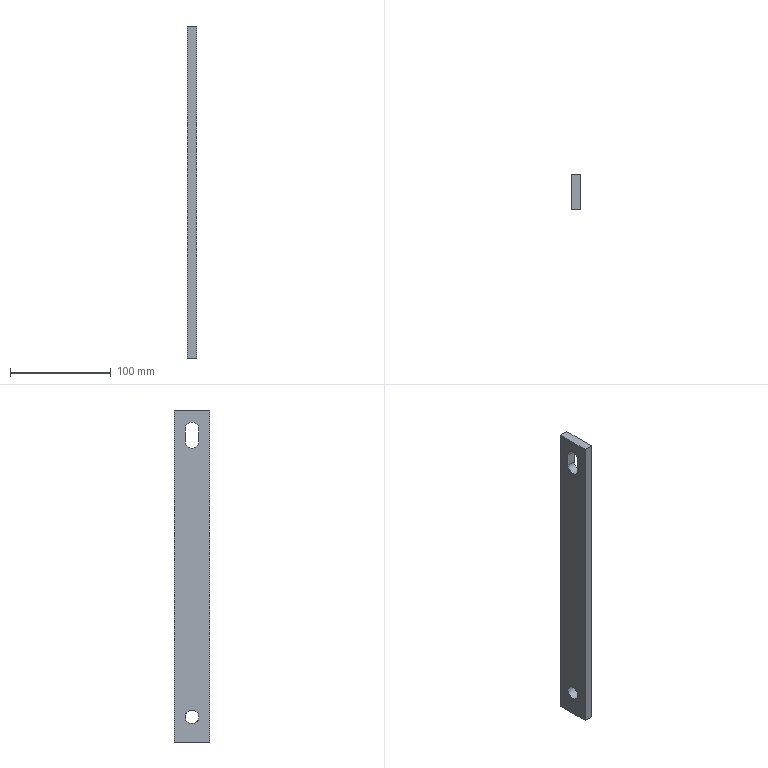Part | NX | features solid 2 | 1 solid | 11 faces | box 9 x 35 x 330 mm | volume 99855 mm3 | plane 8 | cylinder 3 | commonest cylinder face diameters 13.5 x3
STEP:
#1=CARTESIAN_POINT('',(1555.,-656.75,71.25));
#2=VERTEX_POINT('',#1);
#3=CARTESIAN_POINT('',(1555.,-643.25,71.25));
#4=VERTEX_POINT('',#3);
#5=CARTESIAN_POINT('',(1555.,-650.,71.25));
#6=DIRECTION('',(-1.,0.,0.));
#7=DIRECTION('',(0.,0.,-1.));
#8=AXIS2_PLACEMENT_3D('',#5,#6,#7);
#9=CIRCLE('',#8,6.75);
#10=EDGE_CURVE('',#2,#4,#9,.T.);
#11=ORIENTED_EDGE('',*,*,#10,.T.);
#12=CARTESIAN_POINT('',(1564.,-643.25,71.25));
#13=VERTEX_POINT('',#12);
#14=CARTESIAN_POINT('',(1558.,-643.25,71.25));
#15=DIRECTION('',(-1.,0.,0.));
#16=VECTOR('',#15,1000.);
#17=LINE('',#14,#16);
#18=EDGE_CURVE('',#13,#4,#17,.T.);
#19=ORIENTED_EDGE('',*,*,#18,.F.);
#20=CARTESIAN_POINT('',(1564.,-656.75,71.25));
#21=VERTEX_POINT('',#20);
#22=CARTESIAN_POINT('',(1564.,-650.,71.25));
#23=DIRECTION('',(-1.,0.,0.));
#24=DIRECTION('',(0.,0.,-1.));
#25=AXIS2_PLACEMENT_3D('',#22,#23,#24);
#26=CIRCLE('',#25,6.75);
#27=EDGE_CURVE('',#21,#13,#26,.T.);
#28=ORIENTED_EDGE('',*,*,#27,.F.);
#29=CARTESIAN_POINT('',(1558.,-656.75,71.25));
#30=DIRECTION('',(-1.,0.,0.));
#31=VECTOR('',#30,1000.);
#32=LINE('',#29,#31);
#33=EDGE_CURVE('',#21,#2,#32,.T.);
#34=ORIENTED_EDGE('',*,*,#33,.T.);
#35=EDGE_LOOP('',(#11,#19,#28,#34));
#36=FACE_BOUND('',#35,.T.);
#37=CARTESIAN_POINT('',(1558.,-650.,71.25));
#38=DIRECTION('',(-1.,0.,0.));
#39=DIRECTION('',(0.,-1.,0.));
#40=AXIS2_PLACEMENT_3D('',#37,#38,#39);
#41=CYLINDRICAL_SURFACE('',#40,6.75);
#42=ADVANCED_FACE('',(#36),#41,.F.);
#43=CARTESIAN_POINT('',(1555.,-656.75,58.75));
#44=VERTEX_POINT('',#43);
#45=CARTESIAN_POINT('',(1555.,-656.75,41.25));
#46=DIRECTION('',(0.,0.,-1.));
#47=VECTOR('',#46,1000.);
#48=LINE('',#45,#47);
#49=EDGE_CURVE('',#2,#44,#48,.T.);
#50=ORIENTED_EDGE('',*,*,#49,.F.);
#51=ORIENTED_EDGE('',*,*,#33,.F.);
#52=CARTESIAN_POINT('',(1564.,-656.75,58.75));
#53=VERTEX_POINT('',#52);
#54=CARTESIAN_POINT('',(1564.,-656.75,60.));
#55=DIRECTION('',(0.,0.,-1.));
#56=VECTOR('',#55,1000.);
#57=LINE('',#54,#56);
#58=EDGE_CURVE('',#21,#53,#57,.T.);
#59=ORIENTED_EDGE('',*,*,#58,.T.);
#60=CARTESIAN_POINT('',(1558.,-656.75,58.75));
#61=DIRECTION('',(-1.,0.,0.));
#62=VECTOR('',#61,1000.);
#63=LINE('',#60,#62);
#64=EDGE_CURVE('',#53,#44,#63,.T.);
#65=ORIENTED_EDGE('',*,*,#64,.T.);
#66=EDGE_LOOP('',(#50,#51,#59,#65));
#67=FACE_BOUND('',#66,.T.);
#68=CARTESIAN_POINT('',(1558.,-656.75,71.25));
#69=DIRECTION('',(0.,1.,0.));
#70=DIRECTION('',(-1.,0.,0.));
#71=AXIS2_PLACEMENT_3D('',#68,#69,#70);
#72=PLANE('',#71);
#73=ADVANCED_FACE('',(#67),#72,.T.);
#74=CARTESIAN_POINT('',(1555.,-643.25,58.75));
#75=VERTEX_POINT('',#74);
#76=CARTESIAN_POINT('',(1555.,-650.,58.75));
#77=DIRECTION('',(-1.,0.,0.));
#78=DIRECTION('',(0.,0.,-1.));
#79=AXIS2_PLACEMENT_3D('',#76,#77,#78);
#80=CIRCLE('',#79,6.75);
#81=EDGE_CURVE('',#75,#44,#80,.T.);
#82=ORIENTED_EDGE('',*,*,#81,.T.);
#83=ORIENTED_EDGE('',*,*,#64,.F.);
#84=CARTESIAN_POINT('',(1564.,-643.25,58.75));
#85=VERTEX_POINT('',#84);
#86=CARTESIAN_POINT('',(1564.,-650.,58.75));
#87=DIRECTION('',(-1.,0.,0.));
#88=DIRECTION('',(0.,0.,-1.));
#89=AXIS2_PLACEMENT_3D('',#86,#87,#88);
#90=CIRCLE('',#89,6.75);
#91=EDGE_CURVE('',#85,#53,#90,.T.);
#92=ORIENTED_EDGE('',*,*,#91,.F.);
#93=CARTESIAN_POINT('',(1558.,-643.25,58.75));
#94=DIRECTION('',(-1.,0.,0.));
#95=VECTOR('',#94,1000.);
#96=LINE('',#93,#95);
#97=EDGE_CURVE('',#85,#75,#96,.T.);
#98=ORIENTED_EDGE('',*,*,#97,.T.);
#99=EDGE_LOOP('',(#82,#83,#92,#98));
#100=FACE_BOUND('',#99,.T.);
#101=CARTESIAN_POINT('',(1558.,-650.,58.75));
#102=DIRECTION('',(-1.,0.,0.));
#103=DIRECTION('',(0.,-1.,0.));
#104=AXIS2_PLACEMENT_3D('',#101,#102,#103);
#105=CYLINDRICAL_SURFACE('',#104,6.75);
#106=ADVANCED_FACE('',(#100),#105,.F.);
#107=CARTESIAN_POINT('',(1555.,-667.5,-240.));
#108=VERTEX_POINT('',#107);
#109=CARTESIAN_POINT('',(1555.,-667.5,90.));
#110=VERTEX_POINT('',#109);
#111=CARTESIAN_POINT('',(1555.,-667.5,-240.));
#112=DIRECTION('',(0.,0.,1.));
#113=VECTOR('',#112,1000.);
#114=LINE('',#111,#113);
#115=EDGE_CURVE('',#108,#110,#114,.T.);
#116=ORIENTED_EDGE('',*,*,#115,.F.);
#117=CARTESIAN_POINT('',(1564.,-667.5,-240.));
#118=VERTEX_POINT('',#117);
#119=CARTESIAN_POINT('',(1558.,-667.5,-240.));
#120=DIRECTION('',(-1.,0.,0.));
#121=VECTOR('',#120,1000.);
#122=LINE('',#119,#121);
#123=EDGE_CURVE('',#118,#108,#122,.T.);
#124=ORIENTED_EDGE('',*,*,#123,.F.);
#125=CARTESIAN_POINT('',(1564.,-667.5,90.));
#126=VERTEX_POINT('',#125);
#127=CARTESIAN_POINT('',(1564.,-667.5,60.));
#128=DIRECTION('',(0.,0.,1.));
#129=VECTOR('',#128,1000.);
#130=LINE('',#127,#129);
#131=EDGE_CURVE('',#118,#126,#130,.T.);
#132=ORIENTED_EDGE('',*,*,#131,.T.);
#133=CARTESIAN_POINT('',(1558.,-667.5,90.));
#134=DIRECTION('',(-1.,0.,0.));
#135=VECTOR('',#134,1000.);
#136=LINE('',#133,#135);
#137=EDGE_CURVE('',#126,#110,#136,.T.);
#138=ORIENTED_EDGE('',*,*,#137,.T.);
#139=EDGE_LOOP('',(#116,#124,#132,#138));
#140=FACE_BOUND('',#139,.T.);
#141=CARTESIAN_POINT('',(1558.,-667.5,-240.));
#142=DIRECTION('',(0.,-1.,0.));
#143=DIRECTION('',(0.,0.,1.));
#144=AXIS2_PLACEMENT_3D('',#141,#142,#143);
#145=PLANE('',#144);
#146=ADVANCED_FACE('',(#140),#145,.T.);
#147=CARTESIAN_POINT('',(1555.,-632.5,90.));
#148=VERTEX_POINT('',#147);
#149=CARTESIAN_POINT('',(1555.,-667.5,90.));
#150=DIRECTION('',(0.,1.,0.));
#151=VECTOR('',#150,1000.);
#152=LINE('',#149,#151);
#153=EDGE_CURVE('',#110,#148,#152,.T.);
#154=ORIENTED_EDGE('',*,*,#153,.F.);
#155=ORIENTED_EDGE('',*,*,#137,.F.);
#156=CARTESIAN_POINT('',(1564.,-632.5,90.));
#157=VERTEX_POINT('',#156);
#158=CARTESIAN_POINT('',(1564.,-667.5,90.));
#159=DIRECTION('',(0.,1.,0.));
#160=VECTOR('',#159,1000.);
#161=LINE('',#158,#160);
#162=EDGE_CURVE('',#126,#157,#161,.T.);
#163=ORIENTED_EDGE('',*,*,#162,.T.);
#164=CARTESIAN_POINT('',(1558.,-632.5,90.));
#165=DIRECTION('',(-1.,0.,0.));
#166=VECTOR('',#165,1000.);
#167=LINE('',#164,#166);
#168=EDGE_CURVE('',#157,#148,#167,.T.);
#169=ORIENTED_EDGE('',*,*,#168,.T.);
#170=EDGE_LOOP('',(#154,#155,#163,#169));
#171=FACE_BOUND('',#170,.T.);
#172=CARTESIAN_POINT('',(1558.,-667.5,90.));
#173=DIRECTION('',(0.,0.,1.));
#174=DIRECTION('',(-1.,0.,0.));
#175=AXIS2_PLACEMENT_3D('',#172,#173,#174);
#176=PLANE('',#175);
#177=ADVANCED_FACE('',(#171),#176,.T.);
#178=CARTESIAN_POINT('',(1555.,-632.5,-240.));
#179=VERTEX_POINT('',#178);
#180=CARTESIAN_POINT('',(1555.,-632.5,60.));
#181=DIRECTION('',(0.,0.,-1.));
#182=VECTOR('',#181,1000.);
#183=LINE('',#180,#182);
#184=EDGE_CURVE('',#148,#179,#183,.T.);
#185=ORIENTED_EDGE('',*,*,#184,.F.);
#186=ORIENTED_EDGE('',*,*,#168,.F.);
#187=CARTESIAN_POINT('',(1564.,-632.5,-240.));
#188=VERTEX_POINT('',#187);
#189=CARTESIAN_POINT('',(1564.,-632.5,60.));
#190=DIRECTION('',(0.,0.,-1.));
#191=VECTOR('',#190,1000.);
#192=LINE('',#189,#191);
#193=EDGE_CURVE('',#157,#188,#192,.T.);
#194=ORIENTED_EDGE('',*,*,#193,.T.);
#195=CARTESIAN_POINT('',(1558.,-632.5,-240.));
#196=DIRECTION('',(-1.,0.,0.));
#197=VECTOR('',#196,1000.);
#198=LINE('',#195,#197);
#199=EDGE_CURVE('',#188,#179,#198,.T.);
#200=ORIENTED_EDGE('',*,*,#199,.T.);
#201=EDGE_LOOP('',(#185,#186,#194,#200));
#202=FACE_BOUND('',#201,.T.);
#203=CARTESIAN_POINT('',(1558.,-632.5,60.));
#204=DIRECTION('',(0.,1.,0.));
#205=DIRECTION('',(0.,0.,-1.));
#206=AXIS2_PLACEMENT_3D('',#203,#204,#205);
#207=PLANE('',#206);
#208=ADVANCED_FACE('',(#202),#207,.T.);
#209=CARTESIAN_POINT('',(1564.,-650.,-208.25));
#210=VERTEX_POINT('',#209);
#211=CARTESIAN_POINT('',(1564.,-650.,-215.));
#212=DIRECTION('',(-1.,0.,0.));
#213=DIRECTION('',(0.,0.,1.));
#214=AXIS2_PLACEMENT_3D('',#211,#212,#213);
#215=CIRCLE('',#214,6.75);
#216=EDGE_CURVE('',#210,#210,#215,.T.);
#217=ORIENTED_EDGE('',*,*,#216,.F.);
#218=EDGE_LOOP('',(#217));
#219=FACE_BOUND('',#218,.T.);
#220=CARTESIAN_POINT('',(1555.,-656.75,-215.));
#221=VERTEX_POINT('',#220);
#222=CARTESIAN_POINT('',(1555.,-650.,-215.));
#223=DIRECTION('',(-1.,0.,0.));
#224=DIRECTION('',(0.,-1.,0.));
#225=AXIS2_PLACEMENT_3D('',#222,#223,#224);
#226=CIRCLE('',#225,6.75);
#227=EDGE_CURVE('',#221,#221,#226,.T.);
#228=ORIENTED_EDGE('',*,*,#227,.T.);
#229=EDGE_LOOP('',(#228));
#230=FACE_BOUND('',#229,.T.);
#231=CARTESIAN_POINT('',(1558.,-650.,-215.));
#232=DIRECTION('',(-1.,0.,0.));
#233=DIRECTION('',(0.,-1.,0.));
#234=AXIS2_PLACEMENT_3D('',#231,#232,#233);
#235=CYLINDRICAL_SURFACE('',#234,6.75);
#236=ADVANCED_FACE('',(#219,#230),#235,.F.);
#237=CARTESIAN_POINT('',(1555.,-632.5,-240.));
#238=DIRECTION('',(0.,-1.,0.));
#239=VECTOR('',#238,1000.);
#240=LINE('',#237,#239);
#241=EDGE_CURVE('',#179,#108,#240,.T.);
#242=ORIENTED_EDGE('',*,*,#241,.F.);
#243=ORIENTED_EDGE('',*,*,#199,.F.);
#244=CARTESIAN_POINT('',(1564.,-667.5,-240.));
#245=DIRECTION('',(0.,-1.,0.));
#246=VECTOR('',#245,1000.);
#247=LINE('',#244,#246);
#248=EDGE_CURVE('',#188,#118,#247,.T.);
#249=ORIENTED_EDGE('',*,*,#248,.T.);
#250=ORIENTED_EDGE('',*,*,#123,.T.);
#251=EDGE_LOOP('',(#242,#243,#249,#250));
#252=FACE_BOUND('',#251,.T.);
#253=CARTESIAN_POINT('',(1558.,-632.5,-240.));
#254=DIRECTION('',(0.,0.,-1.));
#255=DIRECTION('',(1.,0.,0.));
#256=AXIS2_PLACEMENT_3D('',#253,#254,#255);
#257=PLANE('',#256);
#258=ADVANCED_FACE('',(#252),#257,.T.);
#259=CARTESIAN_POINT('',(1555.,-643.25,28.75));
#260=DIRECTION('',(0.,0.,1.));
#261=VECTOR('',#260,1000.);
#262=LINE('',#259,#261);
#263=EDGE_CURVE('',#75,#4,#262,.T.);
#264=ORIENTED_EDGE('',*,*,#263,.F.);
#265=ORIENTED_EDGE('',*,*,#97,.F.);
#266=CARTESIAN_POINT('',(1564.,-643.25,60.));
#267=DIRECTION('',(0.,0.,1.));
#268=VECTOR('',#267,1000.);
#269=LINE('',#266,#268);
#270=EDGE_CURVE('',#85,#13,#269,.T.);
#271=ORIENTED_EDGE('',*,*,#270,.T.);
#272=ORIENTED_EDGE('',*,*,#18,.T.);
#273=EDGE_LOOP('',(#264,#265,#271,#272));
#274=FACE_BOUND('',#273,.T.);
#275=CARTESIAN_POINT('',(1558.,-643.25,58.75));
#276=DIRECTION('',(0.,-1.,0.));
#277=DIRECTION('',(1.,0.,0.));
#278=AXIS2_PLACEMENT_3D('',#275,#276,#277);
#279=PLANE('',#278);
#280=ADVANCED_FACE('',(#274),#279,.T.);
#281=ORIENTED_EDGE('',*,*,#131,.F.);
#282=ORIENTED_EDGE('',*,*,#248,.F.);
#283=ORIENTED_EDGE('',*,*,#193,.F.);
#284=ORIENTED_EDGE('',*,*,#162,.F.);
#285=EDGE_LOOP('',(#281,#282,#283,#284));
#286=FACE_BOUND('',#285,.T.);
#287=ORIENTED_EDGE('',*,*,#216,.T.);
#288=EDGE_LOOP('',(#287));
#289=FACE_BOUND('',#288,.T.);
#290=ORIENTED_EDGE('',*,*,#27,.T.);
#291=ORIENTED_EDGE('',*,*,#270,.F.);
#292=ORIENTED_EDGE('',*,*,#91,.T.);
#293=ORIENTED_EDGE('',*,*,#58,.F.);
#294=EDGE_LOOP('',(#290,#291,#292,#293));
#295=FACE_BOUND('',#294,.T.);
#296=CARTESIAN_POINT('',(1564.,-667.5,60.));
#297=DIRECTION('',(-1.,0.,0.));
#298=DIRECTION('',(0.,-1.,0.));
#299=AXIS2_PLACEMENT_3D('',#296,#297,#298);
#300=PLANE('',#299);
#301=ADVANCED_FACE('',(#286,#289,#295),#300,.F.);
#302=ORIENTED_EDGE('',*,*,#115,.T.);
#303=ORIENTED_EDGE('',*,*,#153,.T.);
#304=ORIENTED_EDGE('',*,*,#184,.T.);
#305=ORIENTED_EDGE('',*,*,#241,.T.);
#306=EDGE_LOOP('',(#302,#303,#304,#305));
#307=FACE_BOUND('',#306,.T.);
#308=ORIENTED_EDGE('',*,*,#227,.F.);
#309=EDGE_LOOP('',(#308));
#310=FACE_BOUND('',#309,.T.);
#311=ORIENTED_EDGE('',*,*,#10,.F.);
#312=ORIENTED_EDGE('',*,*,#49,.T.);
#313=ORIENTED_EDGE('',*,*,#81,.F.);
#314=ORIENTED_EDGE('',*,*,#263,.T.);
#315=EDGE_LOOP('',(#311,#312,#313,#314));
#316=FACE_BOUND('',#315,.T.);
#317=CARTESIAN_POINT('',(1555.,-667.5,60.));
#318=DIRECTION('',(-1.,0.,0.));
#319=DIRECTION('',(0.,-1.,0.));
#320=AXIS2_PLACEMENT_3D('',#317,#318,#319);
#321=PLANE('',#320);
#322=ADVANCED_FACE('',(#307,#310,#316),#321,.T.);
#323=CLOSED_SHELL('',(#42,#73,#106,#146,#177,#208,#236,#258,#280,#301,#322));
#324=MANIFOLD_SOLID_BREP('',#323);
#325=(LENGTH_UNIT()NAMED_UNIT(*)SI_UNIT(.MILLI.,.METRE.));
#326=UNCERTAINTY_MEASURE_WITH_UNIT(LENGTH_MEASURE(0.00001),#325,'','');
#327=(NAMED_UNIT(*)PLANE_ANGLE_UNIT()SI_UNIT($,.RADIAN.));
#328=(NAMED_UNIT(*)SI_UNIT($,.STERADIAN.)SOLID_ANGLE_UNIT());
#329=(GEOMETRIC_REPRESENTATION_CONTEXT(3)GLOBAL_UNCERTAINTY_ASSIGNED_CONTEXT((#326))GLOBAL_UNIT_ASSIGNED_CONTEXT((#325,#327,#328))REPRESENTATION_CONTEXT('',''));
#330=ADVANCED_BREP_SHAPE_REPRESENTATION('',(#324),#329);